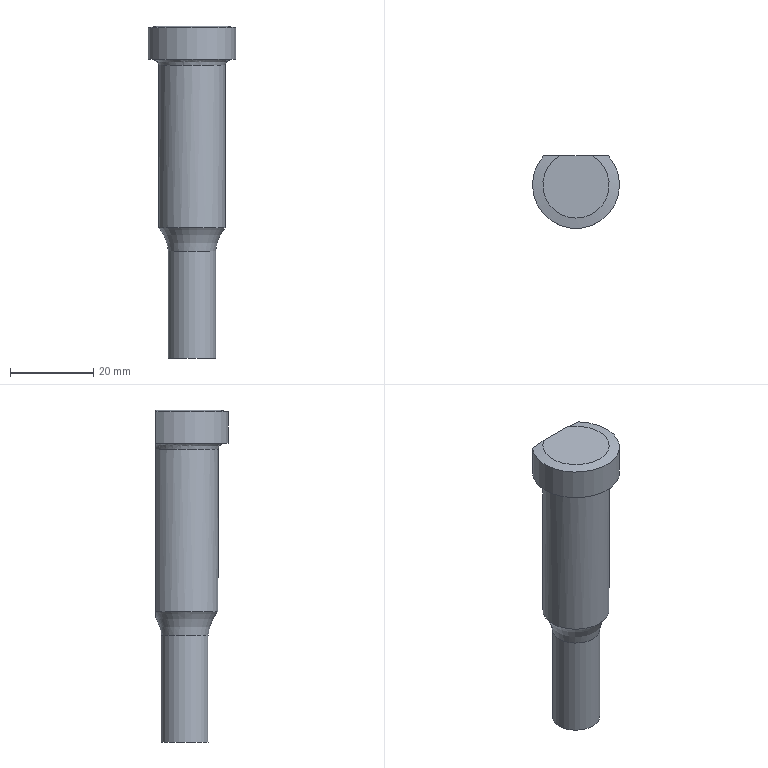Part | NX | features MI_APAL_0252 2 | 1 solid | 10 faces | box 21 x 17.5 x 80 mm | volume 13786 mm3 | plane 4 | cylinder 3 | torus 1 | spline 1 | cone 1 | commonest cylinder face diameters 11.38 x1 16 x1 21 x1
STEP:
#1=CARTESIAN_POINT('',(1379.389,141.904,-40.));
#2=VERTEX_POINT('',#1);
#3=CARTESIAN_POINT('',(1385.079,141.904,-40.));
#4=DIRECTION('',(0.,0.,-1.));
#5=DIRECTION('',(-1.,0.,0.));
#6=AXIS2_PLACEMENT_3D('',#3,#4,#5);
#7=CIRCLE('',#6,5.69);
#8=EDGE_CURVE('',#2,#2,#7,.T.);
#9=ORIENTED_EDGE('',*,*,#8,.T.);
#10=EDGE_LOOP('',(#9));
#11=FACE_BOUND('',#10,.T.);
#12=CARTESIAN_POINT('',(1398.108,153.679,-40.));
#13=DIRECTION('',(0.,0.,-1.));
#14=DIRECTION('',(-1.,0.,0.));
#15=AXIS2_PLACEMENT_3D('',#12,#13,#14);
#16=PLANE('',#15);
#17=ADVANCED_FACE('',(#11),#16,.T.);
#18=CARTESIAN_POINT('',(1379.389,141.904,-14.293));
#19=VERTEX_POINT('',#18);
#20=CARTESIAN_POINT('',(1385.079,141.904,-14.293));
#21=DIRECTION('',(0.,0.,-1.));
#22=DIRECTION('',(-1.,0.,0.));
#23=AXIS2_PLACEMENT_3D('',#20,#21,#22);
#24=CIRCLE('',#23,5.69);
#25=EDGE_CURVE('',#19,#19,#24,.T.);
#26=ORIENTED_EDGE('',*,*,#25,.F.);
#27=CARTESIAN_POINT('',(1377.079,141.904,-8.577));
#28=VERTEX_POINT('',#27);
#29=CARTESIAN_POINT('',(1379.414,141.904,-15.));
#30=CARTESIAN_POINT('',(1379.414,141.904,-11.364));
#31=CARTESIAN_POINT('',(1377.078,141.904,-8.577));
#32=(BOUNDED_CURVE()B_SPLINE_CURVE(2,(#29,#30,#31),.UNSPECIFIED.,.F.,.F.)B_SPLINE_CURVE_WITH_KNOTS((3,3),(0.,0.9999),.UNSPECIFIED.)CURVE()GEOMETRIC_REPRESENTATION_ITEM()RATIONAL_B_SPLINE_CURVE((1.,0.9398,1.))REPRESENTATION_ITEM(''));
#33=EDGE_CURVE('',#19,#28,#32,.T.);
#34=ORIENTED_EDGE('',*,*,#33,.T.);
#35=CARTESIAN_POINT('',(1381.206,148.904,-8.578));
#36=VERTEX_POINT('',#35);
#37=CARTESIAN_POINT('',(1385.079,141.904,-8.578));
#38=DIRECTION('',(0.,0.,-1.));
#39=DIRECTION('',(0.4841,0.875,0.));
#40=AXIS2_PLACEMENT_3D('',#37,#38,#39);
#41=CIRCLE('',#40,8.);
#42=EDGE_CURVE('',#28,#36,#41,.T.);
#43=ORIENTED_EDGE('',*,*,#42,.T.);
#44=CARTESIAN_POINT('',(1388.952,148.904,-8.578));
#45=VERTEX_POINT('',#44);
#46=CARTESIAN_POINT('',(1381.206,148.904,-8.578));
#47=CARTESIAN_POINT('',(1381.551,148.904,-8.778));
#48=CARTESIAN_POINT('',(1382.133,148.904,-9.105));
#49=CARTESIAN_POINT('',(1383.426,148.904,-9.747));
#50=CARTESIAN_POINT('',(1385.079,148.904,-10.182));
#51=CARTESIAN_POINT('',(1386.731,148.904,-9.747));
#52=CARTESIAN_POINT('',(1388.025,148.904,-9.105));
#53=CARTESIAN_POINT('',(1388.605,148.904,-8.778));
#54=CARTESIAN_POINT('',(1388.952,148.904,-8.578));
#55=B_SPLINE_CURVE_WITH_KNOTS('',3,(#46,#47,#48,#49,#50,#51,#52,#53,#54),.UNSPECIFIED.,.F.,.F.,(4,1,1,1,1,1,4),(0.,0.125,0.25,0.5,0.75,0.875,1.),.UNSPECIFIED.);
#56=EDGE_CURVE('',#45,#36,#55,.F.);
#57=ORIENTED_EDGE('',*,*,#56,.F.);
#58=CARTESIAN_POINT('',(1385.079,141.904,-8.578));
#59=DIRECTION('',(0.,0.,-1.));
#60=DIRECTION('',(0.4841,0.875,0.));
#61=AXIS2_PLACEMENT_3D('',#58,#59,#60);
#62=CIRCLE('',#61,8.);
#63=EDGE_CURVE('',#45,#28,#62,.T.);
#64=ORIENTED_EDGE('',*,*,#63,.T.);
#65=ORIENTED_EDGE('',*,*,#33,.F.);
#66=EDGE_LOOP('',(#26,#34,#43,#57,#64,#65));
#67=FACE_BOUND('',#66,.T.);
#68=CARTESIAN_POINT('',(1385.079,141.904,-15.));
#69=DIRECTION('',(0.,0.,-1.));
#70=DIRECTION('',(-1.,0.,0.));
#71=AXIS2_PLACEMENT_3D('',#68,#69,#70);
#72=TOROIDAL_SURFACE('',#71,15.665,10.);
#73=ADVANCED_FACE('',(#67),#72,.F.);
#74=ORIENTED_EDGE('',*,*,#8,.F.);
#75=EDGE_LOOP('',(#74));
#76=FACE_BOUND('',#75,.T.);
#77=ORIENTED_EDGE('',*,*,#25,.T.);
#78=EDGE_LOOP('',(#77));
#79=FACE_BOUND('',#78,.T.);
#80=CARTESIAN_POINT('',(1385.079,141.904,-27.5));
#81=DIRECTION('',(0.,0.,-1.));
#82=DIRECTION('',(-1.,0.,0.));
#83=AXIS2_PLACEMENT_3D('',#80,#81,#82);
#84=CYLINDRICAL_SURFACE('',#83,5.69);
#85=ADVANCED_FACE('',(#76,#79),#84,.T.);
#86=CARTESIAN_POINT('',(1388.952,148.904,40.));
#87=VERTEX_POINT('',#86);
#88=CARTESIAN_POINT('',(1392.905,148.904,39.559));
#89=VERTEX_POINT('',#88);
#90=CARTESIAN_POINT('',(1388.952,148.904,40.));
#91=CARTESIAN_POINT('',(1390.661,148.904,39.854));
#92=CARTESIAN_POINT('',(1392.905,148.904,39.559));
#93=(BOUNDED_CURVE()B_SPLINE_CURVE(2,(#90,#91,#92),.UNSPECIFIED.,.F.,.F.)B_SPLINE_CURVE_WITH_KNOTS((3,3),(0.,3.978),.UNSPECIFIED.)CURVE()GEOMETRIC_REPRESENTATION_ITEM()RATIONAL_B_SPLINE_CURVE((1.,1.024,1.))REPRESENTATION_ITEM(''));
#94=EDGE_CURVE('',#87,#89,#93,.T.);
#95=ORIENTED_EDGE('',*,*,#94,.T.);
#96=CARTESIAN_POINT('',(1392.905,148.904,32.));
#97=VERTEX_POINT('',#96);
#98=CARTESIAN_POINT('',(1392.905,148.904,39.559));
#99=DIRECTION('',(0.,0.,-1.));
#100=VECTOR('',#99,1000.);
#101=LINE('',#98,#100);
#102=EDGE_CURVE('',#89,#97,#101,.T.);
#103=ORIENTED_EDGE('',*,*,#102,.T.);
#104=CARTESIAN_POINT('',(1391.501,148.904,32.));
#105=VERTEX_POINT('',#104);
#106=CARTESIAN_POINT('',(1392.905,148.904,32.));
#107=DIRECTION('',(-1.,0.,0.));
#108=VECTOR('',#107,1000.);
#109=LINE('',#106,#108);
#110=EDGE_CURVE('',#97,#105,#109,.T.);
#111=ORIENTED_EDGE('',*,*,#110,.T.);
#112=CARTESIAN_POINT('',(1388.952,148.904,30.5));
#113=VERTEX_POINT('',#112);
#114=CARTESIAN_POINT('',(1391.501,148.904,32.));
#115=CARTESIAN_POINT('',(1391.34,148.904,32.));
#116=CARTESIAN_POINT('',(1391.164,148.904,31.987));
#117=CARTESIAN_POINT('',(1390.815,148.904,31.935));
#118=CARTESIAN_POINT('',(1390.642,148.904,31.896));
#119=CARTESIAN_POINT('',(1390.341,148.904,31.807));
#120=CARTESIAN_POINT('',(1390.184,148.904,31.75));
#121=CARTESIAN_POINT('',(1389.88,148.904,31.612));
#122=CARTESIAN_POINT('',(1389.734,148.904,31.532));
#123=CARTESIAN_POINT('',(1389.513,148.904,31.385));
#124=CARTESIAN_POINT('',(1389.414,148.904,31.309));
#125=CARTESIAN_POINT('',(1389.234,148.904,31.14));
#126=CARTESIAN_POINT('',(1389.154,148.904,31.047));
#127=CARTESIAN_POINT('',(1389.072,148.904,30.917));
#128=CARTESIAN_POINT('',(1389.05,148.904,30.879));
#129=CARTESIAN_POINT('',(1389.012,148.904,30.799));
#130=CARTESIAN_POINT('',(1388.997,148.904,30.758));
#131=CARTESIAN_POINT('',(1388.975,148.904,30.686));
#132=CARTESIAN_POINT('',(1388.966,148.904,30.649));
#133=CARTESIAN_POINT('',(1388.954,148.904,30.573));
#134=CARTESIAN_POINT('',(1388.952,148.904,30.535));
#135=CARTESIAN_POINT('',(1388.952,148.904,30.5));
#136=B_SPLINE_CURVE_WITH_KNOTS('',3,(#114,#115,#116,#117,#118,#119,#120,#121,#122,#123,#124,#125,#126,#127,#128,#129,#130,#131,#132,#133,#134,#135),.UNSPECIFIED.,.F.,.F.,(4,2,2,2,2,2,2,2,2,2,4),(2.666,3.15,3.633,4.09,4.547,4.887,5.227,5.347,5.467,5.572,5.677),.UNSPECIFIED.);
#137=EDGE_CURVE('',#105,#113,#136,.T.);
#138=ORIENTED_EDGE('',*,*,#137,.T.);
#139=CARTESIAN_POINT('',(1388.952,148.904,30.5));
#140=DIRECTION('',(0.,0.,-1.));
#141=VECTOR('',#140,1000.);
#142=LINE('',#139,#141);
#143=EDGE_CURVE('',#113,#45,#142,.T.);
#144=ORIENTED_EDGE('',*,*,#143,.T.);
#145=ORIENTED_EDGE('',*,*,#56,.T.);
#146=CARTESIAN_POINT('',(1381.206,148.904,30.5));
#147=VERTEX_POINT('',#146);
#148=CARTESIAN_POINT('',(1381.206,148.904,-8.578));
#149=DIRECTION('',(0.,0.,1.));
#150=VECTOR('',#149,1000.);
#151=LINE('',#148,#150);
#152=EDGE_CURVE('',#36,#147,#151,.T.);
#153=ORIENTED_EDGE('',*,*,#152,.T.);
#154=CARTESIAN_POINT('',(1378.656,148.904,32.));
#155=VERTEX_POINT('',#154);
#156=CARTESIAN_POINT('',(1381.206,148.904,30.5));
#157=CARTESIAN_POINT('',(1381.206,148.904,30.535));
#158=CARTESIAN_POINT('',(1381.203,148.904,30.573));
#159=CARTESIAN_POINT('',(1381.191,148.904,30.649));
#160=CARTESIAN_POINT('',(1381.183,148.904,30.686));
#161=CARTESIAN_POINT('',(1381.161,148.904,30.758));
#162=CARTESIAN_POINT('',(1381.145,148.904,30.799));
#163=CARTESIAN_POINT('',(1381.108,148.904,30.879));
#164=CARTESIAN_POINT('',(1381.086,148.904,30.917));
#165=CARTESIAN_POINT('',(1381.004,148.904,31.047));
#166=CARTESIAN_POINT('',(1380.923,148.904,31.14));
#167=CARTESIAN_POINT('',(1380.744,148.904,31.309));
#168=CARTESIAN_POINT('',(1380.645,148.904,31.385));
#169=CARTESIAN_POINT('',(1380.424,148.904,31.532));
#170=CARTESIAN_POINT('',(1380.277,148.904,31.612));
#171=CARTESIAN_POINT('',(1379.973,148.904,31.75));
#172=CARTESIAN_POINT('',(1379.816,148.904,31.807));
#173=CARTESIAN_POINT('',(1379.515,148.904,31.896));
#174=CARTESIAN_POINT('',(1379.343,148.904,31.935));
#175=CARTESIAN_POINT('',(1378.994,148.904,31.987));
#176=CARTESIAN_POINT('',(1378.817,148.904,32.));
#177=CARTESIAN_POINT('',(1378.656,148.904,32.));
#178=B_SPLINE_CURVE_WITH_KNOTS('',3,(#156,#157,#158,#159,#160,#161,#162,#163,#164,#165,#166,#167,#168,#169,#170,#171,#172,#173,#174,#175,#176,#177),.UNSPECIFIED.,.F.,.F.,(4,2,2,2,2,2,2,2,2,2,4),(-5.677,-5.572,-5.467,-5.347,-5.227,-4.887,-4.547,-4.09,-3.633,-3.15,-2.666),.UNSPECIFIED.);
#179=EDGE_CURVE('',#147,#155,#178,.T.);
#180=ORIENTED_EDGE('',*,*,#179,.T.);
#181=CARTESIAN_POINT('',(1377.253,148.904,32.));
#182=VERTEX_POINT('',#181);
#183=CARTESIAN_POINT('',(1378.656,148.904,32.));
#184=DIRECTION('',(-1.,0.,0.));
#185=VECTOR('',#184,1000.);
#186=LINE('',#183,#185);
#187=EDGE_CURVE('',#155,#182,#186,.T.);
#188=ORIENTED_EDGE('',*,*,#187,.T.);
#189=CARTESIAN_POINT('',(1377.253,148.904,39.559));
#190=VERTEX_POINT('',#189);
#191=CARTESIAN_POINT('',(1377.253,148.904,32.));
#192=DIRECTION('',(0.,0.,1.));
#193=VECTOR('',#192,1000.);
#194=LINE('',#191,#193);
#195=EDGE_CURVE('',#182,#190,#194,.T.);
#196=ORIENTED_EDGE('',*,*,#195,.T.);
#197=CARTESIAN_POINT('',(1381.206,148.904,40.));
#198=VERTEX_POINT('',#197);
#199=CARTESIAN_POINT('',(1377.253,148.904,39.559));
#200=CARTESIAN_POINT('',(1379.496,148.904,39.854));
#201=CARTESIAN_POINT('',(1381.206,148.904,40.));
#202=(BOUNDED_CURVE()B_SPLINE_CURVE(2,(#199,#200,#201),.UNSPECIFIED.,.F.,.F.)B_SPLINE_CURVE_WITH_KNOTS((3,3),(0.,3.978),.UNSPECIFIED.)CURVE()GEOMETRIC_REPRESENTATION_ITEM()RATIONAL_B_SPLINE_CURVE((1.,1.024,1.))REPRESENTATION_ITEM(''));
#203=EDGE_CURVE('',#190,#198,#202,.T.);
#204=ORIENTED_EDGE('',*,*,#203,.T.);
#205=CARTESIAN_POINT('',(1381.206,148.904,40.));
#206=DIRECTION('',(1.,0.,0.));
#207=VECTOR('',#206,1000.);
#208=LINE('',#205,#207);
#209=EDGE_CURVE('',#198,#87,#208,.T.);
#210=ORIENTED_EDGE('',*,*,#209,.T.);
#211=EDGE_LOOP('',(#95,#103,#111,#138,#144,#145,#153,#180,#188,#196,#204,#210));
#212=FACE_BOUND('',#211,.T.);
#213=CARTESIAN_POINT('',(1394.47,148.904,45.001));
#214=DIRECTION('',(0.,1.,0.));
#215=DIRECTION('',(-1.,0.,0.));
#216=AXIS2_PLACEMENT_3D('',#213,#214,#215);
#217=PLANE('',#216);
#218=ADVANCED_FACE('',(#212),#217,.T.);
#219=ORIENTED_EDGE('',*,*,#152,.F.);
#220=ORIENTED_EDGE('',*,*,#42,.F.);
#221=ORIENTED_EDGE('',*,*,#63,.F.);
#222=ORIENTED_EDGE('',*,*,#143,.F.);
#223=CARTESIAN_POINT('',(1385.079,141.904,30.5));
#224=DIRECTION('',(0.,0.,-1.));
#225=DIRECTION('',(0.4841,0.875,0.));
#226=AXIS2_PLACEMENT_3D('',#223,#224,#225);
#227=CIRCLE('',#226,8.);
#228=EDGE_CURVE('',#113,#147,#227,.T.);
#229=ORIENTED_EDGE('',*,*,#228,.T.);
#230=EDGE_LOOP('',(#219,#220,#221,#222,#229));
#231=FACE_BOUND('',#230,.T.);
#232=CARTESIAN_POINT('',(1385.079,141.904,8.5));
#233=DIRECTION('',(0.,0.,-1.));
#234=DIRECTION('',(0.008727,1.,0.));
#235=AXIS2_PLACEMENT_3D('',#232,#233,#234);
#236=CYLINDRICAL_SURFACE('',#235,8.);
#237=ADVANCED_FACE('',(#231),#236,.T.);
#238=ORIENTED_EDGE('',*,*,#179,.F.);
#239=ORIENTED_EDGE('',*,*,#228,.F.);
#240=ORIENTED_EDGE('',*,*,#137,.F.);
#241=CARTESIAN_POINT('',(1385.079,141.904,32.));
#242=DIRECTION('',(0.,0.,1.));
#243=DIRECTION('',(-0.6761,0.7368,0.));
#244=AXIS2_PLACEMENT_3D('',#241,#242,#243);
#245=CIRCLE('',#244,9.5);
#246=EDGE_CURVE('',#155,#105,#245,.T.);
#247=ORIENTED_EDGE('',*,*,#246,.F.);
#248=EDGE_LOOP('',(#238,#239,#240,#247));
#249=FACE_BOUND('',#248,.T.);
#250=CARTESIAN_POINT('',(1384.983,152.904,30.5));
#251=CARTESIAN_POINT('',(1395.982,153.,30.5));
#252=CARTESIAN_POINT('',(1396.078,142.,30.5));
#253=CARTESIAN_POINT('',(1396.174,131.,30.5));
#254=CARTESIAN_POINT('',(1385.175,130.904,30.5));
#255=CARTESIAN_POINT('',(1374.175,130.808,30.5));
#256=CARTESIAN_POINT('',(1374.079,141.808,30.5));
#257=CARTESIAN_POINT('',(1373.983,152.808,30.5));
#258=CARTESIAN_POINT('',(1384.983,152.904,30.5));
#259=CARTESIAN_POINT('',(1384.983,152.904,31.366));
#260=CARTESIAN_POINT('',(1395.982,153.,31.366));
#261=CARTESIAN_POINT('',(1396.078,142.,31.366));
#262=CARTESIAN_POINT('',(1396.174,131.,31.366));
#263=CARTESIAN_POINT('',(1385.175,130.904,31.366));
#264=CARTESIAN_POINT('',(1374.175,130.808,31.366));
#265=CARTESIAN_POINT('',(1374.079,141.808,31.366));
#266=CARTESIAN_POINT('',(1373.983,152.808,31.366));
#267=CARTESIAN_POINT('',(1384.983,152.904,31.366));
#268=CARTESIAN_POINT('',(1384.989,152.154,31.799));
#269=CARTESIAN_POINT('',(1395.239,152.243,31.799));
#270=CARTESIAN_POINT('',(1395.328,141.993,31.799));
#271=CARTESIAN_POINT('',(1395.418,131.744,31.799));
#272=CARTESIAN_POINT('',(1385.168,131.654,31.799));
#273=CARTESIAN_POINT('',(1374.919,131.565,31.799));
#274=CARTESIAN_POINT('',(1374.829,141.815,31.799));
#275=CARTESIAN_POINT('',(1374.74,152.064,31.799));
#276=CARTESIAN_POINT('',(1384.989,152.154,31.799));
#277=CARTESIAN_POINT('',(1384.996,151.404,32.232));
#278=CARTESIAN_POINT('',(1394.495,151.487,32.232));
#279=CARTESIAN_POINT('',(1394.578,141.987,32.232));
#280=CARTESIAN_POINT('',(1394.661,132.487,32.232));
#281=CARTESIAN_POINT('',(1385.162,132.404,32.232));
#282=CARTESIAN_POINT('',(1375.662,132.321,32.232));
#283=CARTESIAN_POINT('',(1375.579,141.821,32.232));
#284=CARTESIAN_POINT('',(1375.496,151.321,32.232));
#285=CARTESIAN_POINT('',(1384.996,151.404,32.232));
#286=CARTESIAN_POINT('',(1385.002,150.654,31.799));
#287=CARTESIAN_POINT('',(1393.752,150.73,31.799));
#288=CARTESIAN_POINT('',(1393.828,141.98,31.799));
#289=CARTESIAN_POINT('',(1393.905,133.231,31.799));
#290=CARTESIAN_POINT('',(1385.155,133.154,31.799));
#291=CARTESIAN_POINT('',(1376.406,133.078,31.799));
#292=CARTESIAN_POINT('',(1376.329,141.828,31.799));
#293=CARTESIAN_POINT('',(1376.253,150.577,31.799));
#294=CARTESIAN_POINT('',(1385.002,150.654,31.799));
#295=CARTESIAN_POINT('',(1385.009,149.904,31.366));
#296=CARTESIAN_POINT('',(1393.008,149.973,31.366));
#297=CARTESIAN_POINT('',(1393.078,141.974,31.366));
#298=CARTESIAN_POINT('',(1393.148,133.974,31.366));
#299=CARTESIAN_POINT('',(1385.149,133.904,31.366));
#300=CARTESIAN_POINT('',(1377.149,133.835,31.366));
#301=CARTESIAN_POINT('',(1377.079,141.834,31.366));
#302=CARTESIAN_POINT('',(1377.009,149.834,31.366));
#303=CARTESIAN_POINT('',(1385.009,149.904,31.366));
#304=CARTESIAN_POINT('',(1385.009,149.904,30.5));
#305=CARTESIAN_POINT('',(1393.009,149.974,30.5));
#306=CARTESIAN_POINT('',(1393.078,141.974,30.5));
#307=CARTESIAN_POINT('',(1393.148,133.974,30.5));
#308=CARTESIAN_POINT('',(1385.149,133.904,30.5));
#309=CARTESIAN_POINT('',(1377.149,133.835,30.5));
#310=CARTESIAN_POINT('',(1377.079,141.834,30.5));
#311=CARTESIAN_POINT('',(1377.009,149.834,30.5));
#312=CARTESIAN_POINT('',(1385.009,149.904,30.5));
#313=(BOUNDED_SURFACE()B_SPLINE_SURFACE(2,2,((#250,#251,#252,#253,#254,#255,#256,#257,#258),(#259,#260,#261,#262,#263,#264,#265,#266,#267),(#268,#269,#270,#271,#272,#273,#274,#275,#276),(#277,#278,#279,#280,#281,#282,#283,#284,#285),(#286,#287,#288,#289,#290,#291,#292,#293,#294),(#295,#296,#297,#298,#299,#300,#301,#302,#303),(#304,#305,#306,#307,#308,#309,#310,#311,#312)),.TOROIDAL_SURF.,.F.,.T.,.F.)B_SPLINE_SURFACE_WITH_KNOTS((3,2,2,3),(3,2,2,2,3),(-0.0001752,1.047,2.094,3.142),(0.,1.571,3.142,4.712,6.283),.PIECEWISE_BEZIER_KNOTS.)GEOMETRIC_REPRESENTATION_ITEM()RATIONAL_B_SPLINE_SURFACE(((1.,0.7071,1.,0.7071,1.,0.7071,1.,0.7071,1.),(0.866,0.6124,0.866,0.6124,0.866,0.6124,0.866,0.6124,0.866),(1.,0.7071,1.,0.7071,1.,0.7071,1.,0.7071,1.),(0.866,0.6124,0.866,0.6124,0.866,0.6124,0.866,0.6124,0.866),(1.,0.7071,1.,0.7071,1.,0.7071,1.,0.7071,1.),(0.866,0.6124,0.866,0.6124,0.866,0.6124,0.866,0.6124,0.866),(1.,0.7071,1.,0.7071,1.,0.7071,1.,0.7071,1.)))REPRESENTATION_ITEM('')SURFACE());
#314=ADVANCED_FACE('',(#249),#313,.F.);
#315=ORIENTED_EDGE('',*,*,#187,.F.);
#316=ORIENTED_EDGE('',*,*,#246,.T.);
#317=ORIENTED_EDGE('',*,*,#110,.F.);
#318=CARTESIAN_POINT('',(1385.079,141.904,32.));
#319=DIRECTION('',(0.,0.,1.));
#320=DIRECTION('',(-0.7454,0.6667,0.));
#321=AXIS2_PLACEMENT_3D('',#318,#319,#320);
#322=CIRCLE('',#321,10.5);
#323=EDGE_CURVE('',#182,#97,#322,.T.);
#324=ORIENTED_EDGE('',*,*,#323,.F.);
#325=EDGE_LOOP('',(#315,#316,#317,#324));
#326=FACE_BOUND('',#325,.T.);
#327=CARTESIAN_POINT('',(1402.564,151.062,32.));
#328=DIRECTION('',(0.,0.,-1.));
#329=DIRECTION('',(-1.,0.,0.));
#330=AXIS2_PLACEMENT_3D('',#327,#328,#329);
#331=PLANE('',#330);
#332=ADVANCED_FACE('',(#326),#331,.T.);
#333=ORIENTED_EDGE('',*,*,#195,.F.);
#334=ORIENTED_EDGE('',*,*,#323,.T.);
#335=ORIENTED_EDGE('',*,*,#102,.F.);
#336=CARTESIAN_POINT('',(1385.079,141.904,39.559));
#337=DIRECTION('',(0.,0.,-1.));
#338=DIRECTION('',(0.7454,0.6667,0.));
#339=AXIS2_PLACEMENT_3D('',#336,#337,#338);
#340=CIRCLE('',#339,10.5);
#341=EDGE_CURVE('',#89,#190,#340,.T.);
#342=ORIENTED_EDGE('',*,*,#341,.T.);
#343=EDGE_LOOP('',(#333,#334,#335,#342));
#344=FACE_BOUND('',#343,.T.);
#345=CARTESIAN_POINT('',(1385.079,141.904,36.));
#346=DIRECTION('',(0.,0.,-1.));
#347=DIRECTION('',(0.008727,1.,0.));
#348=AXIS2_PLACEMENT_3D('',#345,#346,#347);
#349=CYLINDRICAL_SURFACE('',#348,10.5);
#350=ADVANCED_FACE('',(#344),#349,.T.);
#351=ORIENTED_EDGE('',*,*,#209,.F.);
#352=CARTESIAN_POINT('',(1385.079,141.904,40.));
#353=DIRECTION('',(0.,0.,1.));
#354=DIRECTION('',(-0.4841,0.875,0.));
#355=AXIS2_PLACEMENT_3D('',#352,#353,#354);
#356=CIRCLE('',#355,8.);
#357=EDGE_CURVE('',#198,#87,#356,.T.);
#358=ORIENTED_EDGE('',*,*,#357,.T.);
#359=EDGE_LOOP('',(#351,#358));
#360=FACE_BOUND('',#359,.T.);
#361=CARTESIAN_POINT('',(1370.296,150.858,40.));
#362=DIRECTION('',(0.,0.,1.));
#363=DIRECTION('',(1.,0.,0.));
#364=AXIS2_PLACEMENT_3D('',#361,#362,#363);
#365=PLANE('',#364);
#366=ADVANCED_FACE('',(#360),#365,.T.);
#367=ORIENTED_EDGE('',*,*,#203,.F.);
#368=ORIENTED_EDGE('',*,*,#341,.F.);
#369=ORIENTED_EDGE('',*,*,#94,.F.);
#370=ORIENTED_EDGE('',*,*,#357,.F.);
#371=EDGE_LOOP('',(#367,#368,#369,#370));
#372=FACE_BOUND('',#371,.T.);
#373=CARTESIAN_POINT('',(1385.079,141.904,38.792));
#374=DIRECTION('',(0.,0.,-1.));
#375=DIRECTION('',(-0.008727,1.,0.));
#376=AXIS2_PLACEMENT_3D('',#373,#374,#375);
#377=CONICAL_SURFACE('',#376,14.849,1.396);
#378=ADVANCED_FACE('',(#372),#377,.T.);
#379=CLOSED_SHELL('',(#17,#73,#85,#218,#237,#314,#332,#350,#366,#378));
#380=MANIFOLD_SOLID_BREP('',#379);
#381=(LENGTH_UNIT()NAMED_UNIT(*)SI_UNIT(.MILLI.,.METRE.));
#382=UNCERTAINTY_MEASURE_WITH_UNIT(LENGTH_MEASURE(0.0508),#381,'','');
#383=(NAMED_UNIT(*)PLANE_ANGLE_UNIT()SI_UNIT($,.RADIAN.));
#384=(NAMED_UNIT(*)SI_UNIT($,.STERADIAN.)SOLID_ANGLE_UNIT());
#385=(GEOMETRIC_REPRESENTATION_CONTEXT(3)GLOBAL_UNCERTAINTY_ASSIGNED_CONTEXT((#382))GLOBAL_UNIT_ASSIGNED_CONTEXT((#381,#383,#384))REPRESENTATION_CONTEXT('',''));
#386=ADVANCED_BREP_SHAPE_REPRESENTATION('',(#380),#385);